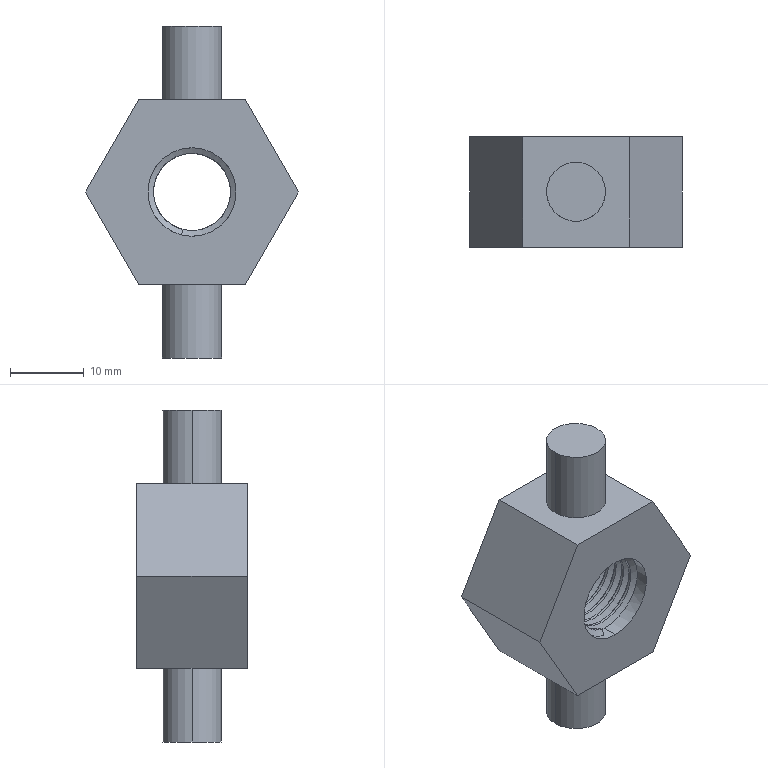Part | SolidWorks | features Extrusion 1, ICE 1, MirrorPattern 1, SweepThread 1 | 1 solid | 39 faces | box 28.868 x 15 x 45 mm | volume 7627 mm3 | cylinder 24 | plane 12 | spline 3 | commonest cylinder face diameters 12 x20 8 x4